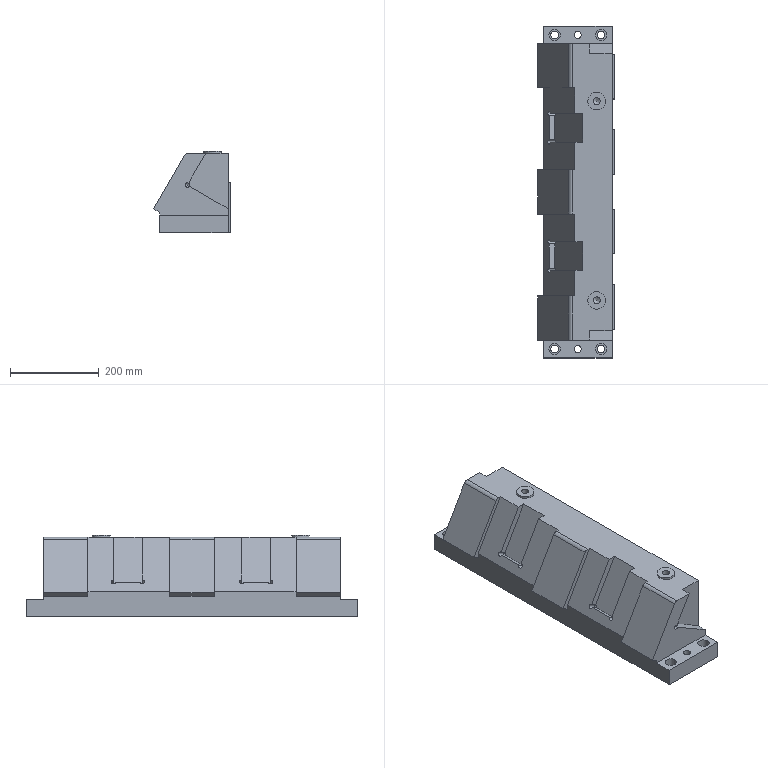Part | NX | features solid 2 | 1 solid | 127 faces | box 173.349 x 750 x 185 mm | volume 11956571 mm3 | plane 92 | cylinder 23 | cone 8 | spline 4 | commonest cylinder face diameters 10 x6 16 x4 17.5 x4 25.5 x4 20 x3 40 x2